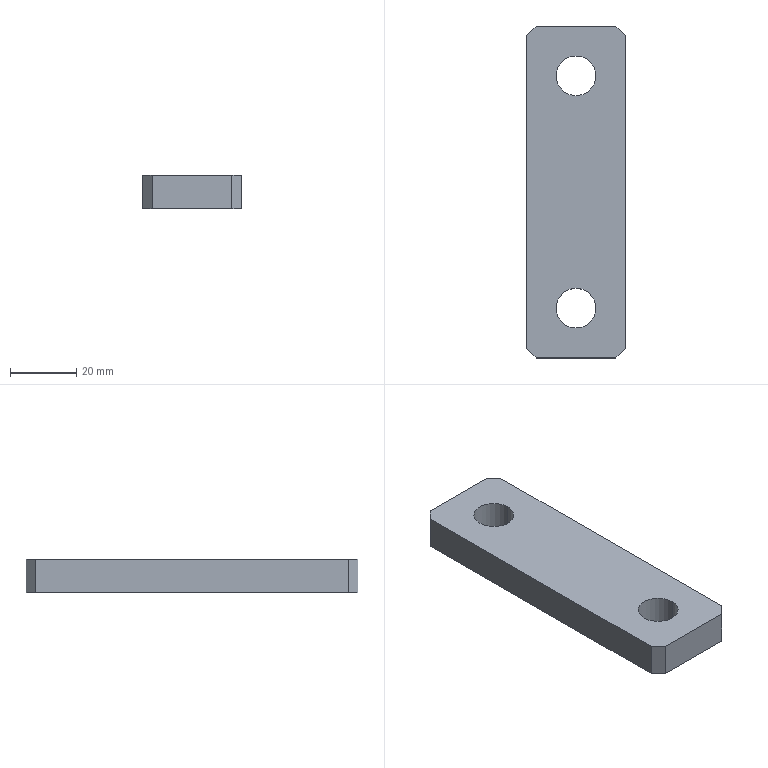Part | STEP file | 1 solid | 14 faces | box 30 x 100 x 10 mm | volume 27558 mm3 | plane 10 | cylinder 4 | commonest cylinder face diameters 12 x4
STEP:
#1=CARTESIAN_POINT('',(0.,0.,0.));
#2=DIRECTION('',(0.,0.,1.));
#3=DIRECTION('',(1.,0.,0.));
#4=AXIS2_PLACEMENT_3D('',#1,#2,#3);
#5=CARTESIAN_POINT('',(-6.,35.,5.));
#6=VERTEX_POINT('',#5);
#7=CARTESIAN_POINT('',(-6.,35.,-5.));
#8=VERTEX_POINT('',#7);
#9=CARTESIAN_POINT('',(-6.,35.,-5.));
#10=DIRECTION('',(0.,0.,-1.));
#11=VECTOR('',#10,1.);
#12=LINE('',#9,#11);
#13=CARTESIAN_POINT('',(0.,35.,-5.));
#14=DIRECTION('',(0.,0.,-1.));
#15=DIRECTION('',(-1.,0.,0.));
#16=AXIS2_PLACEMENT_3D('',#13,#14,#15);
#17=CYLINDRICAL_SURFACE('',#16,6.);
#18=CARTESIAN_POINT('',(6.283,0.));
#19=DIRECTION('',(0.,1.));
#20=VECTOR('',#19,1.);
#21=LINE('',#18,#20);
#22=(GEOMETRIC_REPRESENTATION_CONTEXT(2)PARAMETRIC_REPRESENTATION_CONTEXT()REPRESENTATION_CONTEXT('',''));
#23=DEFINITIONAL_REPRESENTATION('',(#21),#22);
#24=PCURVE('',#17,#23);
#25=CARTESIAN_POINT('',(0.,35.,-5.));
#26=DIRECTION('',(0.,0.,-1.));
#27=DIRECTION('',(-1.,0.,0.));
#28=AXIS2_PLACEMENT_3D('',#25,#26,#27);
#29=CYLINDRICAL_SURFACE('',#28,6.);
#30=CARTESIAN_POINT('',(0.,0.));
#31=DIRECTION('',(0.,1.));
#32=VECTOR('',#31,1.);
#33=LINE('',#30,#32);
#34=(GEOMETRIC_REPRESENTATION_CONTEXT(2)PARAMETRIC_REPRESENTATION_CONTEXT()REPRESENTATION_CONTEXT('',''));
#35=DEFINITIONAL_REPRESENTATION('',(#33),#34);
#36=PCURVE('',#29,#35);
#37=SURFACE_CURVE('',#12,(#24,#36),.PCURVE_S1.);
#38=EDGE_CURVE('',#6,#8,#37,.T.);
#39=ORIENTED_EDGE('',*,*,#38,.T.);
#40=CARTESIAN_POINT('',(6.,35.,-5.));
#41=VERTEX_POINT('',#40);
#42=CARTESIAN_POINT('',(0.,35.,-5.));
#43=DIRECTION('',(0.,0.,1.));
#44=DIRECTION('',(-1.,0.,0.));
#45=AXIS2_PLACEMENT_3D('',#42,#43,#44);
#46=CIRCLE('',#45,6.);
#47=CARTESIAN_POINT('',(6.283,0.));
#48=DIRECTION('',(-1.,0.));
#49=VECTOR('',#48,1.);
#50=LINE('',#47,#49);
#51=(GEOMETRIC_REPRESENTATION_CONTEXT(2)PARAMETRIC_REPRESENTATION_CONTEXT()REPRESENTATION_CONTEXT('',''));
#52=DEFINITIONAL_REPRESENTATION('',(#50),#51);
#53=PCURVE('',#17,#52);
#54=CARTESIAN_POINT('',(0.,0.,-5.));
#55=DIRECTION('',(0.,0.,1.));
#56=DIRECTION('',(1.,0.,0.));
#57=AXIS2_PLACEMENT_3D('',#54,#55,#56);
#58=PLANE('',#57);
#59=CARTESIAN_POINT('',(0.,35.));
#60=DIRECTION('',(-1.,0.));
#61=AXIS2_PLACEMENT_2D('',#59,#60);
#62=CIRCLE('',#61,6.);
#63=(GEOMETRIC_REPRESENTATION_CONTEXT(2)PARAMETRIC_REPRESENTATION_CONTEXT()REPRESENTATION_CONTEXT('',''));
#64=DEFINITIONAL_REPRESENTATION('',(#62),#63);
#65=PCURVE('',#58,#64);
#66=SURFACE_CURVE('',#46,(#53,#65),.PCURVE_S1.);
#67=EDGE_CURVE('',#8,#41,#66,.T.);
#68=ORIENTED_EDGE('',*,*,#67,.T.);
#69=CARTESIAN_POINT('',(6.,35.,5.));
#70=VERTEX_POINT('',#69);
#71=CARTESIAN_POINT('',(6.,35.,-5.));
#72=DIRECTION('',(0.,0.,-1.));
#73=VECTOR('',#72,1.);
#74=LINE('',#71,#73);
#75=CARTESIAN_POINT('',(3.142,0.));
#76=DIRECTION('',(0.,1.));
#77=VECTOR('',#76,1.);
#78=LINE('',#75,#77);
#79=(GEOMETRIC_REPRESENTATION_CONTEXT(2)PARAMETRIC_REPRESENTATION_CONTEXT()REPRESENTATION_CONTEXT('',''));
#80=DEFINITIONAL_REPRESENTATION('',(#78),#79);
#81=PCURVE('',#17,#80);
#82=CARTESIAN_POINT('',(3.142,0.));
#83=DIRECTION('',(0.,1.));
#84=VECTOR('',#83,1.);
#85=LINE('',#82,#84);
#86=(GEOMETRIC_REPRESENTATION_CONTEXT(2)PARAMETRIC_REPRESENTATION_CONTEXT()REPRESENTATION_CONTEXT('',''));
#87=DEFINITIONAL_REPRESENTATION('',(#85),#86);
#88=PCURVE('',#29,#87);
#89=SURFACE_CURVE('',#74,(#81,#88),.PCURVE_S1.);
#90=EDGE_CURVE('',#70,#41,#89,.T.);
#91=ORIENTED_EDGE('',*,*,#90,.F.);
#92=CARTESIAN_POINT('',(0.,35.,5.));
#93=DIRECTION('',(0.,0.,-1.));
#94=DIRECTION('',(-1.,0.,0.));
#95=AXIS2_PLACEMENT_3D('',#92,#93,#94);
#96=CIRCLE('',#95,6.);
#97=CARTESIAN_POINT('',(0.,-10.));
#98=DIRECTION('',(1.,0.));
#99=VECTOR('',#98,1.);
#100=LINE('',#97,#99);
#101=(GEOMETRIC_REPRESENTATION_CONTEXT(2)PARAMETRIC_REPRESENTATION_CONTEXT()REPRESENTATION_CONTEXT('',''));
#102=DEFINITIONAL_REPRESENTATION('',(#100),#101);
#103=PCURVE('',#17,#102);
#104=CARTESIAN_POINT('',(0.,0.,5.));
#105=DIRECTION('',(0.,0.,1.));
#106=DIRECTION('',(1.,0.,0.));
#107=AXIS2_PLACEMENT_3D('',#104,#105,#106);
#108=PLANE('',#107);
#109=CARTESIAN_POINT('',(-6.,35.));
#110=CARTESIAN_POINT('',(-6.,45.392));
#111=CARTESIAN_POINT('',(3.,40.196));
#112=CARTESIAN_POINT('',(12.,35.));
#113=CARTESIAN_POINT('',(3.,29.804));
#114=CARTESIAN_POINT('',(-6.,24.608));
#115=CARTESIAN_POINT('',(-6.,35.));
#116=(BOUNDED_CURVE()B_SPLINE_CURVE(2,(#109,#110,#111,#112,#113,#114,#115),.UNSPECIFIED.,.T.,.F.)B_SPLINE_CURVE_WITH_KNOTS((1,2,2,2,2,1),(-2.094,0.,2.094,4.189,6.283,8.378),.UNSPECIFIED.)CURVE()GEOMETRIC_REPRESENTATION_ITEM()RATIONAL_B_SPLINE_CURVE((1.,0.5,1.,0.5,1.,0.5,1.))REPRESENTATION_ITEM(''));
#117=(GEOMETRIC_REPRESENTATION_CONTEXT(2)PARAMETRIC_REPRESENTATION_CONTEXT()REPRESENTATION_CONTEXT('',''));
#118=DEFINITIONAL_REPRESENTATION('',(#116),#117);
#119=PCURVE('',#108,#118);
#120=SURFACE_CURVE('',#96,(#103,#119),.PCURVE_S1.);
#121=EDGE_CURVE('',#70,#6,#120,.T.);
#122=ORIENTED_EDGE('',*,*,#121,.T.);
#123=EDGE_LOOP('',(#39,#68,#91,#122));
#124=FACE_BOUND('',#123,.F.);
#125=ADVANCED_FACE('',(#124),#17,.F.);
#126=CARTESIAN_POINT('',(-6.,-35.,5.));
#127=VERTEX_POINT('',#126);
#128=CARTESIAN_POINT('',(-6.,-35.,-5.));
#129=VERTEX_POINT('',#128);
#130=CARTESIAN_POINT('',(-6.,-35.,-5.));
#131=DIRECTION('',(0.,0.,-1.));
#132=VECTOR('',#131,1.);
#133=LINE('',#130,#132);
#134=CARTESIAN_POINT('',(0.,-35.,-5.));
#135=DIRECTION('',(0.,0.,-1.));
#136=DIRECTION('',(-1.,0.,0.));
#137=AXIS2_PLACEMENT_3D('',#134,#135,#136);
#138=CYLINDRICAL_SURFACE('',#137,6.);
#139=CARTESIAN_POINT('',(6.283,0.));
#140=DIRECTION('',(0.,1.));
#141=VECTOR('',#140,1.);
#142=LINE('',#139,#141);
#143=(GEOMETRIC_REPRESENTATION_CONTEXT(2)PARAMETRIC_REPRESENTATION_CONTEXT()REPRESENTATION_CONTEXT('',''));
#144=DEFINITIONAL_REPRESENTATION('',(#142),#143);
#145=PCURVE('',#138,#144);
#146=CARTESIAN_POINT('',(0.,-35.,-5.));
#147=DIRECTION('',(0.,0.,-1.));
#148=DIRECTION('',(-1.,0.,0.));
#149=AXIS2_PLACEMENT_3D('',#146,#147,#148);
#150=CYLINDRICAL_SURFACE('',#149,6.);
#151=CARTESIAN_POINT('',(0.,0.));
#152=DIRECTION('',(0.,1.));
#153=VECTOR('',#152,1.);
#154=LINE('',#151,#153);
#155=(GEOMETRIC_REPRESENTATION_CONTEXT(2)PARAMETRIC_REPRESENTATION_CONTEXT()REPRESENTATION_CONTEXT('',''));
#156=DEFINITIONAL_REPRESENTATION('',(#154),#155);
#157=PCURVE('',#150,#156);
#158=SURFACE_CURVE('',#133,(#145,#157),.PCURVE_S1.);
#159=EDGE_CURVE('',#127,#129,#158,.T.);
#160=ORIENTED_EDGE('',*,*,#159,.T.);
#161=CARTESIAN_POINT('',(6.,-35.,-5.));
#162=VERTEX_POINT('',#161);
#163=CARTESIAN_POINT('',(0.,-35.,-5.));
#164=DIRECTION('',(0.,0.,1.));
#165=DIRECTION('',(-1.,0.,0.));
#166=AXIS2_PLACEMENT_3D('',#163,#164,#165);
#167=CIRCLE('',#166,6.);
#168=CARTESIAN_POINT('',(6.283,0.));
#169=DIRECTION('',(-1.,0.));
#170=VECTOR('',#169,1.);
#171=LINE('',#168,#170);
#172=(GEOMETRIC_REPRESENTATION_CONTEXT(2)PARAMETRIC_REPRESENTATION_CONTEXT()REPRESENTATION_CONTEXT('',''));
#173=DEFINITIONAL_REPRESENTATION('',(#171),#172);
#174=PCURVE('',#138,#173);
#175=CARTESIAN_POINT('',(0.,-35.));
#176=DIRECTION('',(-1.,0.));
#177=AXIS2_PLACEMENT_2D('',#175,#176);
#178=CIRCLE('',#177,6.);
#179=(GEOMETRIC_REPRESENTATION_CONTEXT(2)PARAMETRIC_REPRESENTATION_CONTEXT()REPRESENTATION_CONTEXT('',''));
#180=DEFINITIONAL_REPRESENTATION('',(#178),#179);
#181=PCURVE('',#58,#180);
#182=SURFACE_CURVE('',#167,(#174,#181),.PCURVE_S1.);
#183=EDGE_CURVE('',#129,#162,#182,.T.);
#184=ORIENTED_EDGE('',*,*,#183,.T.);
#185=CARTESIAN_POINT('',(6.,-35.,5.));
#186=VERTEX_POINT('',#185);
#187=CARTESIAN_POINT('',(6.,-35.,-5.));
#188=DIRECTION('',(0.,0.,-1.));
#189=VECTOR('',#188,1.);
#190=LINE('',#187,#189);
#191=CARTESIAN_POINT('',(3.142,0.));
#192=DIRECTION('',(0.,1.));
#193=VECTOR('',#192,1.);
#194=LINE('',#191,#193);
#195=(GEOMETRIC_REPRESENTATION_CONTEXT(2)PARAMETRIC_REPRESENTATION_CONTEXT()REPRESENTATION_CONTEXT('',''));
#196=DEFINITIONAL_REPRESENTATION('',(#194),#195);
#197=PCURVE('',#138,#196);
#198=CARTESIAN_POINT('',(3.142,0.));
#199=DIRECTION('',(0.,1.));
#200=VECTOR('',#199,1.);
#201=LINE('',#198,#200);
#202=(GEOMETRIC_REPRESENTATION_CONTEXT(2)PARAMETRIC_REPRESENTATION_CONTEXT()REPRESENTATION_CONTEXT('',''));
#203=DEFINITIONAL_REPRESENTATION('',(#201),#202);
#204=PCURVE('',#150,#203);
#205=SURFACE_CURVE('',#190,(#197,#204),.PCURVE_S1.);
#206=EDGE_CURVE('',#186,#162,#205,.T.);
#207=ORIENTED_EDGE('',*,*,#206,.F.);
#208=CARTESIAN_POINT('',(0.,-35.,5.));
#209=DIRECTION('',(0.,0.,-1.));
#210=DIRECTION('',(-1.,0.,0.));
#211=AXIS2_PLACEMENT_3D('',#208,#209,#210);
#212=CIRCLE('',#211,6.);
#213=CARTESIAN_POINT('',(0.,-10.));
#214=DIRECTION('',(1.,0.));
#215=VECTOR('',#214,1.);
#216=LINE('',#213,#215);
#217=(GEOMETRIC_REPRESENTATION_CONTEXT(2)PARAMETRIC_REPRESENTATION_CONTEXT()REPRESENTATION_CONTEXT('',''));
#218=DEFINITIONAL_REPRESENTATION('',(#216),#217);
#219=PCURVE('',#138,#218);
#220=CARTESIAN_POINT('',(-6.,-35.));
#221=CARTESIAN_POINT('',(-6.,-24.608));
#222=CARTESIAN_POINT('',(3.,-29.804));
#223=CARTESIAN_POINT('',(12.,-35.));
#224=CARTESIAN_POINT('',(3.,-40.196));
#225=CARTESIAN_POINT('',(-6.,-45.392));
#226=CARTESIAN_POINT('',(-6.,-35.));
#227=(BOUNDED_CURVE()B_SPLINE_CURVE(2,(#220,#221,#222,#223,#224,#225,#226),.UNSPECIFIED.,.T.,.F.)B_SPLINE_CURVE_WITH_KNOTS((1,2,2,2,2,1),(-2.094,0.,2.094,4.189,6.283,8.378),.UNSPECIFIED.)CURVE()GEOMETRIC_REPRESENTATION_ITEM()RATIONAL_B_SPLINE_CURVE((1.,0.5,1.,0.5,1.,0.5,1.))REPRESENTATION_ITEM(''));
#228=(GEOMETRIC_REPRESENTATION_CONTEXT(2)PARAMETRIC_REPRESENTATION_CONTEXT()REPRESENTATION_CONTEXT('',''));
#229=DEFINITIONAL_REPRESENTATION('',(#227),#228);
#230=PCURVE('',#108,#229);
#231=SURFACE_CURVE('',#212,(#219,#230),.PCURVE_S1.);
#232=EDGE_CURVE('',#186,#127,#231,.T.);
#233=ORIENTED_EDGE('',*,*,#232,.T.);
#234=EDGE_LOOP('',(#160,#184,#207,#233));
#235=FACE_BOUND('',#234,.F.);
#236=ADVANCED_FACE('',(#235),#138,.F.);
#237=CARTESIAN_POINT('',(0.,35.,5.));
#238=DIRECTION('',(0.,0.,-1.));
#239=DIRECTION('',(-1.,0.,0.));
#240=AXIS2_PLACEMENT_3D('',#237,#238,#239);
#241=CIRCLE('',#240,6.);
#242=CARTESIAN_POINT('',(-6.,35.));
#243=CARTESIAN_POINT('',(-6.,45.392));
#244=CARTESIAN_POINT('',(3.,40.196));
#245=CARTESIAN_POINT('',(12.,35.));
#246=CARTESIAN_POINT('',(3.,29.804));
#247=CARTESIAN_POINT('',(-6.,24.608));
#248=CARTESIAN_POINT('',(-6.,35.));
#249=(BOUNDED_CURVE()B_SPLINE_CURVE(2,(#242,#243,#244,#245,#246,#247,#248),.UNSPECIFIED.,.T.,.F.)B_SPLINE_CURVE_WITH_KNOTS((1,2,2,2,2,1),(-2.094,0.,2.094,4.189,6.283,8.378),.UNSPECIFIED.)CURVE()GEOMETRIC_REPRESENTATION_ITEM()RATIONAL_B_SPLINE_CURVE((1.,0.5,1.,0.5,1.,0.5,1.))REPRESENTATION_ITEM(''));
#250=(GEOMETRIC_REPRESENTATION_CONTEXT(2)PARAMETRIC_REPRESENTATION_CONTEXT()REPRESENTATION_CONTEXT('',''));
#251=DEFINITIONAL_REPRESENTATION('',(#249),#250);
#252=PCURVE('',#108,#251);
#253=CARTESIAN_POINT('',(0.,-10.));
#254=DIRECTION('',(1.,0.));
#255=VECTOR('',#254,1.);
#256=LINE('',#253,#255);
#257=(GEOMETRIC_REPRESENTATION_CONTEXT(2)PARAMETRIC_REPRESENTATION_CONTEXT()REPRESENTATION_CONTEXT('',''));
#258=DEFINITIONAL_REPRESENTATION('',(#256),#257);
#259=PCURVE('',#29,#258);
#260=SURFACE_CURVE('',#241,(#252,#259),.PCURVE_S1.);
#261=EDGE_CURVE('',#6,#70,#260,.T.);
#262=ORIENTED_EDGE('',*,*,#261,.T.);
#263=ORIENTED_EDGE('',*,*,#121,.T.);
#264=EDGE_LOOP('',(#262,#263));
#265=FACE_BOUND('',#264,.T.);
#266=CARTESIAN_POINT('',(0.,-35.,5.));
#267=DIRECTION('',(0.,0.,-1.));
#268=DIRECTION('',(-1.,0.,0.));
#269=AXIS2_PLACEMENT_3D('',#266,#267,#268);
#270=CIRCLE('',#269,6.);
#271=CARTESIAN_POINT('',(-6.,-35.));
#272=CARTESIAN_POINT('',(-6.,-24.608));
#273=CARTESIAN_POINT('',(3.,-29.804));
#274=CARTESIAN_POINT('',(12.,-35.));
#275=CARTESIAN_POINT('',(3.,-40.196));
#276=CARTESIAN_POINT('',(-6.,-45.392));
#277=CARTESIAN_POINT('',(-6.,-35.));
#278=(BOUNDED_CURVE()B_SPLINE_CURVE(2,(#271,#272,#273,#274,#275,#276,#277),.UNSPECIFIED.,.T.,.F.)B_SPLINE_CURVE_WITH_KNOTS((1,2,2,2,2,1),(-2.094,0.,2.094,4.189,6.283,8.378),.UNSPECIFIED.)CURVE()GEOMETRIC_REPRESENTATION_ITEM()RATIONAL_B_SPLINE_CURVE((1.,0.5,1.,0.5,1.,0.5,1.))REPRESENTATION_ITEM(''));
#279=(GEOMETRIC_REPRESENTATION_CONTEXT(2)PARAMETRIC_REPRESENTATION_CONTEXT()REPRESENTATION_CONTEXT('',''));
#280=DEFINITIONAL_REPRESENTATION('',(#278),#279);
#281=PCURVE('',#108,#280);
#282=CARTESIAN_POINT('',(0.,-10.));
#283=DIRECTION('',(1.,0.));
#284=VECTOR('',#283,1.);
#285=LINE('',#282,#284);
#286=(GEOMETRIC_REPRESENTATION_CONTEXT(2)PARAMETRIC_REPRESENTATION_CONTEXT()REPRESENTATION_CONTEXT('',''));
#287=DEFINITIONAL_REPRESENTATION('',(#285),#286);
#288=PCURVE('',#150,#287);
#289=SURFACE_CURVE('',#270,(#281,#288),.PCURVE_S1.);
#290=EDGE_CURVE('',#127,#186,#289,.T.);
#291=ORIENTED_EDGE('',*,*,#290,.T.);
#292=ORIENTED_EDGE('',*,*,#232,.T.);
#293=EDGE_LOOP('',(#291,#292));
#294=FACE_BOUND('',#293,.T.);
#295=CARTESIAN_POINT('',(12.,50.,5.));
#296=VERTEX_POINT('',#295);
#297=CARTESIAN_POINT('',(-12.,50.,5.));
#298=VERTEX_POINT('',#297);
#299=CARTESIAN_POINT('',(0.,50.,5.));
#300=DIRECTION('',(-1.,0.,0.));
#301=VECTOR('',#300,1.);
#302=LINE('',#299,#301);
#303=CARTESIAN_POINT('',(0.,50.));
#304=DIRECTION('',(-1.,0.));
#305=VECTOR('',#304,1.);
#306=LINE('',#303,#305);
#307=(GEOMETRIC_REPRESENTATION_CONTEXT(2)PARAMETRIC_REPRESENTATION_CONTEXT()REPRESENTATION_CONTEXT('',''));
#308=DEFINITIONAL_REPRESENTATION('',(#306),#307);
#309=PCURVE('',#108,#308);
#310=CARTESIAN_POINT('',(-15.,50.,5.));
#311=DIRECTION('',(0.,-1.,0.));
#312=DIRECTION('',(0.,0.,-1.));
#313=AXIS2_PLACEMENT_3D('',#310,#311,#312);
#314=PLANE('',#313);
#315=CARTESIAN_POINT('',(0.,15.));
#316=DIRECTION('',(0.,-1.));
#317=VECTOR('',#316,1.);
#318=LINE('',#315,#317);
#319=(GEOMETRIC_REPRESENTATION_CONTEXT(2)PARAMETRIC_REPRESENTATION_CONTEXT()REPRESENTATION_CONTEXT('',''));
#320=DEFINITIONAL_REPRESENTATION('',(#318),#319);
#321=PCURVE('',#314,#320);
#322=SURFACE_CURVE('',#302,(#309,#321),.PCURVE_S1.);
#323=EDGE_CURVE('',#296,#298,#322,.T.);
#324=ORIENTED_EDGE('',*,*,#323,.T.);
#325=CARTESIAN_POINT('',(-15.,47.,5.));
#326=VERTEX_POINT('',#325);
#327=CARTESIAN_POINT('',(-12.,50.,5.));
#328=DIRECTION('',(-0.7071,-0.7071,0.));
#329=VECTOR('',#328,1.);
#330=LINE('',#327,#329);
#331=CARTESIAN_POINT('',(-12.,50.));
#332=DIRECTION('',(-0.7071,-0.7071));
#333=VECTOR('',#332,1.);
#334=LINE('',#331,#333);
#335=(GEOMETRIC_REPRESENTATION_CONTEXT(2)PARAMETRIC_REPRESENTATION_CONTEXT()REPRESENTATION_CONTEXT('',''));
#336=DEFINITIONAL_REPRESENTATION('',(#334),#335);
#337=PCURVE('',#108,#336);
#338=CARTESIAN_POINT('',(-15.,47.,5.));
#339=DIRECTION('',(0.7071,-0.7071,0.));
#340=DIRECTION('',(0.7071,0.7071,0.));
#341=AXIS2_PLACEMENT_3D('',#338,#339,#340);
#342=PLANE('',#341);
#343=CARTESIAN_POINT('',(4.243,0.));
#344=DIRECTION('',(-1.,0.));
#345=VECTOR('',#344,1.);
#346=LINE('',#343,#345);
#347=(GEOMETRIC_REPRESENTATION_CONTEXT(2)PARAMETRIC_REPRESENTATION_CONTEXT()REPRESENTATION_CONTEXT('',''));
#348=DEFINITIONAL_REPRESENTATION('',(#346),#347);
#349=PCURVE('',#342,#348);
#350=SURFACE_CURVE('',#330,(#337,#349),.PCURVE_S1.);
#351=EDGE_CURVE('',#298,#326,#350,.T.);
#352=ORIENTED_EDGE('',*,*,#351,.T.);
#353=CARTESIAN_POINT('',(-15.,-47.,5.));
#354=VERTEX_POINT('',#353);
#355=CARTESIAN_POINT('',(-15.,0.,5.));
#356=DIRECTION('',(0.,-1.,0.));
#357=VECTOR('',#356,1.);
#358=LINE('',#355,#357);
#359=CARTESIAN_POINT('',(-15.,0.));
#360=DIRECTION('',(0.,-1.));
#361=VECTOR('',#360,1.);
#362=LINE('',#359,#361);
#363=(GEOMETRIC_REPRESENTATION_CONTEXT(2)PARAMETRIC_REPRESENTATION_CONTEXT()REPRESENTATION_CONTEXT('',''));
#364=DEFINITIONAL_REPRESENTATION('',(#362),#363);
#365=PCURVE('',#108,#364);
#366=CARTESIAN_POINT('',(-15.,50.,5.));
#367=DIRECTION('',(1.,0.,0.));
#368=DIRECTION('',(0.,1.,0.));
#369=AXIS2_PLACEMENT_3D('',#366,#367,#368);
#370=PLANE('',#369);
#371=CARTESIAN_POINT('',(-50.,0.));
#372=DIRECTION('',(-1.,0.));
#373=VECTOR('',#372,1.);
#374=LINE('',#371,#373);
#375=(GEOMETRIC_REPRESENTATION_CONTEXT(2)PARAMETRIC_REPRESENTATION_CONTEXT()REPRESENTATION_CONTEXT('',''));
#376=DEFINITIONAL_REPRESENTATION('',(#374),#375);
#377=PCURVE('',#370,#376);
#378=SURFACE_CURVE('',#358,(#365,#377),.PCURVE_S1.);
#379=EDGE_CURVE('',#326,#354,#378,.T.);
#380=ORIENTED_EDGE('',*,*,#379,.T.);
#381=CARTESIAN_POINT('',(-12.,-50.,5.));
#382=VERTEX_POINT('',#381);
#383=CARTESIAN_POINT('',(-15.,-47.,5.));
#384=DIRECTION('',(0.7071,-0.7071,0.));
#385=VECTOR('',#384,1.);
#386=LINE('',#383,#385);
#387=CARTESIAN_POINT('',(-15.,-47.));
#388=DIRECTION('',(0.7071,-0.7071));
#389=VECTOR('',#388,1.);
#390=LINE('',#387,#389);
#391=(GEOMETRIC_REPRESENTATION_CONTEXT(2)PARAMETRIC_REPRESENTATION_CONTEXT()REPRESENTATION_CONTEXT('',''));
#392=DEFINITIONAL_REPRESENTATION('',(#390),#391);
#393=PCURVE('',#108,#392);
#394=CARTESIAN_POINT('',(-12.,-50.,5.));
#395=DIRECTION('',(0.7071,0.7071,0.));
#396=DIRECTION('',(-0.7071,0.7071,0.));
#397=AXIS2_PLACEMENT_3D('',#394,#395,#396);
#398=PLANE('',#397);
#399=CARTESIAN_POINT('',(4.243,0.));
#400=DIRECTION('',(-1.,0.));
#401=VECTOR('',#400,1.);
#402=LINE('',#399,#401);
#403=(GEOMETRIC_REPRESENTATION_CONTEXT(2)PARAMETRIC_REPRESENTATION_CONTEXT()REPRESENTATION_CONTEXT('',''));
#404=DEFINITIONAL_REPRESENTATION('',(#402),#403);
#405=PCURVE('',#398,#404);
#406=SURFACE_CURVE('',#386,(#393,#405),.PCURVE_S1.);
#407=EDGE_CURVE('',#354,#382,#406,.T.);
#408=ORIENTED_EDGE('',*,*,#407,.T.);
#409=CARTESIAN_POINT('',(12.,-50.,5.));
#410=VERTEX_POINT('',#409);
#411=CARTESIAN_POINT('',(0.,-50.,5.));
#412=DIRECTION('',(1.,0.,0.));
#413=VECTOR('',#412,1.);
#414=LINE('',#411,#413);
#415=CARTESIAN_POINT('',(0.,-50.));
#416=DIRECTION('',(1.,0.));
#417=VECTOR('',#416,1.);
#418=LINE('',#415,#417);
#419=(GEOMETRIC_REPRESENTATION_CONTEXT(2)PARAMETRIC_REPRESENTATION_CONTEXT()REPRESENTATION_CONTEXT('',''));
#420=DEFINITIONAL_REPRESENTATION('',(#418),#419);
#421=PCURVE('',#108,#420);
#422=CARTESIAN_POINT('',(-15.,-50.,5.));
#423=DIRECTION('',(0.,1.,0.));
#424=DIRECTION('',(0.,0.,1.));
#425=AXIS2_PLACEMENT_3D('',#422,#423,#424);
#426=PLANE('',#425);
#427=CARTESIAN_POINT('',(0.,15.));
#428=DIRECTION('',(0.,1.));
#429=VECTOR('',#428,1.);
#430=LINE('',#427,#429);
#431=(GEOMETRIC_REPRESENTATION_CONTEXT(2)PARAMETRIC_REPRESENTATION_CONTEXT()REPRESENTATION_CONTEXT('',''));
#432=DEFINITIONAL_REPRESENTATION('',(#430),#431);
#433=PCURVE('',#426,#432);
#434=SURFACE_CURVE('',#414,(#421,#433),.PCURVE_S1.);
#435=EDGE_CURVE('',#382,#410,#434,.T.);
#436=ORIENTED_EDGE('',*,*,#435,.T.);
#437=CARTESIAN_POINT('',(15.,-47.,5.));
#438=VERTEX_POINT('',#437);
#439=CARTESIAN_POINT('',(12.,-50.,5.));
#440=DIRECTION('',(0.7071,0.7071,0.));
#441=VECTOR('',#440,1.);
#442=LINE('',#439,#441);
#443=CARTESIAN_POINT('',(12.,-50.));
#444=DIRECTION('',(0.7071,0.7071));
#445=VECTOR('',#444,1.);
#446=LINE('',#443,#445);
#447=(GEOMETRIC_REPRESENTATION_CONTEXT(2)PARAMETRIC_REPRESENTATION_CONTEXT()REPRESENTATION_CONTEXT('',''));
#448=DEFINITIONAL_REPRESENTATION('',(#446),#447);
#449=PCURVE('',#108,#448);
#450=CARTESIAN_POINT('',(15.,-47.,5.));
#451=DIRECTION('',(-0.7071,0.7071,0.));
#452=DIRECTION('',(-0.7071,-0.7071,0.));
#453=AXIS2_PLACEMENT_3D('',#450,#451,#452);
#454=PLANE('',#453);
#455=CARTESIAN_POINT('',(4.243,0.));
#456=DIRECTION('',(-1.,0.));
#457=VECTOR('',#456,1.);
#458=LINE('',#455,#457);
#459=(GEOMETRIC_REPRESENTATION_CONTEXT(2)PARAMETRIC_REPRESENTATION_CONTEXT()REPRESENTATION_CONTEXT('',''));
#460=DEFINITIONAL_REPRESENTATION('',(#458),#459);
#461=PCURVE('',#454,#460);
#462=SURFACE_CURVE('',#442,(#449,#461),.PCURVE_S1.);
#463=EDGE_CURVE('',#410,#438,#462,.T.);
#464=ORIENTED_EDGE('',*,*,#463,.T.);
#465=CARTESIAN_POINT('',(15.,47.,5.));
#466=VERTEX_POINT('',#465);
#467=CARTESIAN_POINT('',(15.,0.,5.));
#468=DIRECTION('',(0.,1.,0.));
#469=VECTOR('',#468,1.);
#470=LINE('',#467,#469);
#471=CARTESIAN_POINT('',(15.,0.));
#472=DIRECTION('',(0.,1.));
#473=VECTOR('',#472,1.);
#474=LINE('',#471,#473);
#475=(GEOMETRIC_REPRESENTATION_CONTEXT(2)PARAMETRIC_REPRESENTATION_CONTEXT()REPRESENTATION_CONTEXT('',''));
#476=DEFINITIONAL_REPRESENTATION('',(#474),#475);
#477=PCURVE('',#108,#476);
#478=CARTESIAN_POINT('',(15.,50.,5.));
#479=DIRECTION('',(-1.,0.,0.));
#480=DIRECTION('',(0.,-1.,0.));
#481=AXIS2_PLACEMENT_3D('',#478,#479,#480);
#482=PLANE('',#481);
#483=CARTESIAN_POINT('',(50.,0.));
#484=DIRECTION('',(-1.,0.));
#485=VECTOR('',#484,1.);
#486=LINE('',#483,#485);
#487=(GEOMETRIC_REPRESENTATION_CONTEXT(2)PARAMETRIC_REPRESENTATION_CONTEXT()REPRESENTATION_CONTEXT('',''));
#488=DEFINITIONAL_REPRESENTATION('',(#486),#487);
#489=PCURVE('',#482,#488);
#490=SURFACE_CURVE('',#470,(#477,#489),.PCURVE_S1.);
#491=EDGE_CURVE('',#438,#466,#490,.T.);
#492=ORIENTED_EDGE('',*,*,#491,.T.);
#493=CARTESIAN_POINT('',(15.,47.,5.));
#494=DIRECTION('',(-0.7071,0.7071,0.));
#495=VECTOR('',#494,1.);
#496=LINE('',#493,#495);
#497=CARTESIAN_POINT('',(15.,47.));
#498=DIRECTION('',(-0.7071,0.7071));
#499=VECTOR('',#498,1.);
#500=LINE('',#497,#499);
#501=(GEOMETRIC_REPRESENTATION_CONTEXT(2)PARAMETRIC_REPRESENTATION_CONTEXT()REPRESENTATION_CONTEXT('',''));
#502=DEFINITIONAL_REPRESENTATION('',(#500),#501);
#503=PCURVE('',#108,#502);
#504=CARTESIAN_POINT('',(12.,50.,5.));
#505=DIRECTION('',(-0.7071,-0.7071,0.));
#506=DIRECTION('',(0.7071,-0.7071,0.));
#507=AXIS2_PLACEMENT_3D('',#504,#505,#506);
#508=PLANE('',#507);
#509=CARTESIAN_POINT('',(4.243,0.));
#510=DIRECTION('',(-1.,0.));
#511=VECTOR('',#510,1.);
#512=LINE('',#509,#511);
#513=(GEOMETRIC_REPRESENTATION_CONTEXT(2)PARAMETRIC_REPRESENTATION_CONTEXT()REPRESENTATION_CONTEXT('',''));
#514=DEFINITIONAL_REPRESENTATION('',(#512),#513);
#515=PCURVE('',#508,#514);
#516=SURFACE_CURVE('',#496,(#503,#515),.PCURVE_S1.);
#517=EDGE_CURVE('',#466,#296,#516,.T.);
#518=ORIENTED_EDGE('',*,*,#517,.T.);
#519=EDGE_LOOP('',(#324,#352,#380,#408,#436,#464,#492,#518));
#520=FACE_BOUND('',#519,.T.);
#521=ADVANCED_FACE('',(#265,#294,#520),#108,.T.);
#522=CARTESIAN_POINT('',(0.,35.,-5.));
#523=DIRECTION('',(0.,0.,1.));
#524=DIRECTION('',(-1.,0.,0.));
#525=AXIS2_PLACEMENT_3D('',#522,#523,#524);
#526=CIRCLE('',#525,6.);
#527=CARTESIAN_POINT('',(6.283,0.));
#528=DIRECTION('',(-1.,0.));
#529=VECTOR('',#528,1.);
#530=LINE('',#527,#529);
#531=(GEOMETRIC_REPRESENTATION_CONTEXT(2)PARAMETRIC_REPRESENTATION_CONTEXT()REPRESENTATION_CONTEXT('',''));
#532=DEFINITIONAL_REPRESENTATION('',(#530),#531);
#533=PCURVE('',#29,#532);
#534=CARTESIAN_POINT('',(0.,35.));
#535=DIRECTION('',(-1.,0.));
#536=AXIS2_PLACEMENT_2D('',#534,#535);
#537=CIRCLE('',#536,6.);
#538=(GEOMETRIC_REPRESENTATION_CONTEXT(2)PARAMETRIC_REPRESENTATION_CONTEXT()REPRESENTATION_CONTEXT('',''));
#539=DEFINITIONAL_REPRESENTATION('',(#537),#538);
#540=PCURVE('',#58,#539);
#541=SURFACE_CURVE('',#526,(#533,#540),.PCURVE_S1.);
#542=EDGE_CURVE('',#41,#8,#541,.T.);
#543=ORIENTED_EDGE('',*,*,#542,.T.);
#544=ORIENTED_EDGE('',*,*,#38,.F.);
#545=ORIENTED_EDGE('',*,*,#261,.T.);
#546=ORIENTED_EDGE('',*,*,#90,.T.);
#547=EDGE_LOOP('',(#543,#544,#545,#546));
#548=FACE_BOUND('',#547,.F.);
#549=ADVANCED_FACE('',(#548),#29,.F.);
#550=CARTESIAN_POINT('',(0.,-35.,-5.));
#551=DIRECTION('',(0.,0.,1.));
#552=DIRECTION('',(-1.,0.,0.));
#553=AXIS2_PLACEMENT_3D('',#550,#551,#552);
#554=CIRCLE('',#553,6.);
#555=CARTESIAN_POINT('',(6.283,0.));
#556=DIRECTION('',(-1.,0.));
#557=VECTOR('',#556,1.);
#558=LINE('',#555,#557);
#559=(GEOMETRIC_REPRESENTATION_CONTEXT(2)PARAMETRIC_REPRESENTATION_CONTEXT()REPRESENTATION_CONTEXT('',''));
#560=DEFINITIONAL_REPRESENTATION('',(#558),#559);
#561=PCURVE('',#150,#560);
#562=CARTESIAN_POINT('',(0.,-35.));
#563=DIRECTION('',(-1.,0.));
#564=AXIS2_PLACEMENT_2D('',#562,#563);
#565=CIRCLE('',#564,6.);
#566=(GEOMETRIC_REPRESENTATION_CONTEXT(2)PARAMETRIC_REPRESENTATION_CONTEXT()REPRESENTATION_CONTEXT('',''));
#567=DEFINITIONAL_REPRESENTATION('',(#565),#566);
#568=PCURVE('',#58,#567);
#569=SURFACE_CURVE('',#554,(#561,#568),.PCURVE_S1.);
#570=EDGE_CURVE('',#162,#129,#569,.T.);
#571=ORIENTED_EDGE('',*,*,#570,.T.);
#572=ORIENTED_EDGE('',*,*,#159,.F.);
#573=ORIENTED_EDGE('',*,*,#290,.T.);
#574=ORIENTED_EDGE('',*,*,#206,.T.);
#575=EDGE_LOOP('',(#571,#572,#573,#574));
#576=FACE_BOUND('',#575,.F.);
#577=ADVANCED_FACE('',(#576),#150,.F.);
#578=CARTESIAN_POINT('',(-12.,50.,-5.));
#579=VERTEX_POINT('',#578);
#580=CARTESIAN_POINT('',(-12.,50.,5.));
#581=DIRECTION('',(0.,0.,1.));
#582=VECTOR('',#581,1.);
#583=LINE('',#580,#582);
#584=CARTESIAN_POINT('',(4.243,0.));
#585=DIRECTION('',(0.,1.));
#586=VECTOR('',#585,1.);
#587=LINE('',#584,#586);
#588=(GEOMETRIC_REPRESENTATION_CONTEXT(2)PARAMETRIC_REPRESENTATION_CONTEXT()REPRESENTATION_CONTEXT('',''));
#589=DEFINITIONAL_REPRESENTATION('',(#587),#588);
#590=PCURVE('',#342,#589);
#591=CARTESIAN_POINT('',(0.,3.));
#592=DIRECTION('',(-1.,0.));
#593=VECTOR('',#592,1.);
#594=LINE('',#591,#593);
#595=(GEOMETRIC_REPRESENTATION_CONTEXT(2)PARAMETRIC_REPRESENTATION_CONTEXT()REPRESENTATION_CONTEXT('',''));
#596=DEFINITIONAL_REPRESENTATION('',(#594),#595);
#597=PCURVE('',#314,#596);
#598=SURFACE_CURVE('',#583,(#590,#597),.PCURVE_S1.);
#599=EDGE_CURVE('',#579,#298,#598,.T.);
#600=ORIENTED_EDGE('',*,*,#599,.F.);
#601=CARTESIAN_POINT('',(-15.,47.,-5.));
#602=VERTEX_POINT('',#601);
#603=CARTESIAN_POINT('',(-15.,47.,-5.));
#604=DIRECTION('',(0.7071,0.7071,0.));
#605=VECTOR('',#604,1.);
#606=LINE('',#603,#605);
#607=CARTESIAN_POINT('',(0.,-10.));
#608=DIRECTION('',(1.,0.));
#609=VECTOR('',#608,1.);
#610=LINE('',#607,#609);
#611=(GEOMETRIC_REPRESENTATION_CONTEXT(2)PARAMETRIC_REPRESENTATION_CONTEXT()REPRESENTATION_CONTEXT('',''));
#612=DEFINITIONAL_REPRESENTATION('',(#610),#611);
#613=PCURVE('',#342,#612);
#614=CARTESIAN_POINT('',(-15.,47.));
#615=DIRECTION('',(0.7071,0.7071));
#616=VECTOR('',#615,1.);
#617=LINE('',#614,#616);
#618=(GEOMETRIC_REPRESENTATION_CONTEXT(2)PARAMETRIC_REPRESENTATION_CONTEXT()REPRESENTATION_CONTEXT('',''));
#619=DEFINITIONAL_REPRESENTATION('',(#617),#618);
#620=PCURVE('',#58,#619);
#621=SURFACE_CURVE('',#606,(#613,#620),.PCURVE_S1.);
#622=EDGE_CURVE('',#602,#579,#621,.T.);
#623=ORIENTED_EDGE('',*,*,#622,.F.);
#624=CARTESIAN_POINT('',(-15.,47.,5.));
#625=DIRECTION('',(0.,0.,-1.));
#626=VECTOR('',#625,1.);
#627=LINE('',#624,#626);
#628=CARTESIAN_POINT('',(0.,0.));
#629=DIRECTION('',(0.,-1.));
#630=VECTOR('',#629,1.);
#631=LINE('',#628,#630);
#632=(GEOMETRIC_REPRESENTATION_CONTEXT(2)PARAMETRIC_REPRESENTATION_CONTEXT()REPRESENTATION_CONTEXT('',''));
#633=DEFINITIONAL_REPRESENTATION('',(#631),#632);
#634=PCURVE('',#342,#633);
#635=CARTESIAN_POINT('',(-3.,0.));
#636=DIRECTION('',(0.,-1.));
#637=VECTOR('',#636,1.);
#638=LINE('',#635,#637);
#639=(GEOMETRIC_REPRESENTATION_CONTEXT(2)PARAMETRIC_REPRESENTATION_CONTEXT()REPRESENTATION_CONTEXT('',''));
#640=DEFINITIONAL_REPRESENTATION('',(#638),#639);
#641=PCURVE('',#370,#640);
#642=SURFACE_CURVE('',#627,(#634,#641),.PCURVE_S1.);
#643=EDGE_CURVE('',#326,#602,#642,.T.);
#644=ORIENTED_EDGE('',*,*,#643,.F.);
#645=ORIENTED_EDGE('',*,*,#351,.F.);
#646=EDGE_LOOP('',(#600,#623,#644,#645));
#647=FACE_BOUND('',#646,.T.);
#648=ADVANCED_FACE('',(#647),#342,.F.);
#649=ORIENTED_EDGE('',*,*,#599,.T.);
#650=ORIENTED_EDGE('',*,*,#323,.F.);
#651=CARTESIAN_POINT('',(12.,50.,-5.));
#652=VERTEX_POINT('',#651);
#653=CARTESIAN_POINT('',(12.,50.,5.));
#654=DIRECTION('',(0.,0.,1.));
#655=VECTOR('',#654,1.);
#656=LINE('',#653,#655);
#657=CARTESIAN_POINT('',(0.,27.));
#658=DIRECTION('',(-1.,0.));
#659=VECTOR('',#658,1.);
#660=LINE('',#657,#659);
#661=(GEOMETRIC_REPRESENTATION_CONTEXT(2)PARAMETRIC_REPRESENTATION_CONTEXT()REPRESENTATION_CONTEXT('',''));
#662=DEFINITIONAL_REPRESENTATION('',(#660),#661);
#663=PCURVE('',#314,#662);
#664=CARTESIAN_POINT('',(0.,0.));
#665=DIRECTION('',(0.,1.));
#666=VECTOR('',#665,1.);
#667=LINE('',#664,#666);
#668=(GEOMETRIC_REPRESENTATION_CONTEXT(2)PARAMETRIC_REPRESENTATION_CONTEXT()REPRESENTATION_CONTEXT('',''));
#669=DEFINITIONAL_REPRESENTATION('',(#667),#668);
#670=PCURVE('',#508,#669);
#671=SURFACE_CURVE('',#656,(#663,#670),.PCURVE_S1.);
#672=EDGE_CURVE('',#652,#296,#671,.T.);
#673=ORIENTED_EDGE('',*,*,#672,.F.);
#674=CARTESIAN_POINT('',(-15.,50.,-5.));
#675=DIRECTION('',(1.,0.,0.));
#676=VECTOR('',#675,1.);
#677=LINE('',#674,#676);
#678=CARTESIAN_POINT('',(10.,0.));
#679=DIRECTION('',(0.,1.));
#680=VECTOR('',#679,1.);
#681=LINE('',#678,#680);
#682=(GEOMETRIC_REPRESENTATION_CONTEXT(2)PARAMETRIC_REPRESENTATION_CONTEXT()REPRESENTATION_CONTEXT('',''));
#683=DEFINITIONAL_REPRESENTATION('',(#681),#682);
#684=PCURVE('',#314,#683);
#685=CARTESIAN_POINT('',(-15.,50.));
#686=DIRECTION('',(1.,0.));
#687=VECTOR('',#686,1.);
#688=LINE('',#685,#687);
#689=(GEOMETRIC_REPRESENTATION_CONTEXT(2)PARAMETRIC_REPRESENTATION_CONTEXT()REPRESENTATION_CONTEXT('',''));
#690=DEFINITIONAL_REPRESENTATION('',(#688),#689);
#691=PCURVE('',#58,#690);
#692=SURFACE_CURVE('',#677,(#684,#691),.PCURVE_S1.);
#693=EDGE_CURVE('',#579,#652,#692,.T.);
#694=ORIENTED_EDGE('',*,*,#693,.F.);
#695=EDGE_LOOP('',(#649,#650,#673,#694));
#696=FACE_BOUND('',#695,.T.);
#697=ADVANCED_FACE('',(#696),#314,.F.);
#698=CARTESIAN_POINT('',(15.,47.,-5.));
#699=VERTEX_POINT('',#698);
#700=CARTESIAN_POINT('',(15.,47.,5.));
#701=DIRECTION('',(0.,0.,1.));
#702=VECTOR('',#701,1.);
#703=LINE('',#700,#702);
#704=CARTESIAN_POINT('',(4.243,0.));
#705=DIRECTION('',(0.,1.));
#706=VECTOR('',#705,1.);
#707=LINE('',#704,#706);
#708=(GEOMETRIC_REPRESENTATION_CONTEXT(2)PARAMETRIC_REPRESENTATION_CONTEXT()REPRESENTATION_CONTEXT('',''));
#709=DEFINITIONAL_REPRESENTATION('',(#707),#708);
#710=PCURVE('',#508,#709);
#711=CARTESIAN_POINT('',(3.,0.));
#712=DIRECTION('',(0.,1.));
#713=VECTOR('',#712,1.);
#714=LINE('',#711,#713);
#715=(GEOMETRIC_REPRESENTATION_CONTEXT(2)PARAMETRIC_REPRESENTATION_CONTEXT()REPRESENTATION_CONTEXT('',''));
#716=DEFINITIONAL_REPRESENTATION('',(#714),#715);
#717=PCURVE('',#482,#716);
#718=SURFACE_CURVE('',#703,(#710,#717),.PCURVE_S1.);
#719=EDGE_CURVE('',#699,#466,#718,.T.);
#720=ORIENTED_EDGE('',*,*,#719,.F.);
#721=CARTESIAN_POINT('',(12.,50.,-5.));
#722=DIRECTION('',(0.7071,-0.7071,0.));
#723=VECTOR('',#722,1.);
#724=LINE('',#721,#723);
#725=CARTESIAN_POINT('',(0.,-10.));
#726=DIRECTION('',(1.,0.));
#727=VECTOR('',#726,1.);
#728=LINE('',#725,#727);
#729=(GEOMETRIC_REPRESENTATION_CONTEXT(2)PARAMETRIC_REPRESENTATION_CONTEXT()REPRESENTATION_CONTEXT('',''));
#730=DEFINITIONAL_REPRESENTATION('',(#728),#729);
#731=PCURVE('',#508,#730);
#732=CARTESIAN_POINT('',(12.,50.));
#733=DIRECTION('',(0.7071,-0.7071));
#734=VECTOR('',#733,1.);
#735=LINE('',#732,#734);
#736=(GEOMETRIC_REPRESENTATION_CONTEXT(2)PARAMETRIC_REPRESENTATION_CONTEXT()REPRESENTATION_CONTEXT('',''));
#737=DEFINITIONAL_REPRESENTATION('',(#735),#736);
#738=PCURVE('',#58,#737);
#739=SURFACE_CURVE('',#724,(#731,#738),.PCURVE_S1.);
#740=EDGE_CURVE('',#652,#699,#739,.T.);
#741=ORIENTED_EDGE('',*,*,#740,.F.);
#742=ORIENTED_EDGE('',*,*,#672,.T.);
#743=ORIENTED_EDGE('',*,*,#517,.F.);
#744=EDGE_LOOP('',(#720,#741,#742,#743));
#745=FACE_BOUND('',#744,.T.);
#746=ADVANCED_FACE('',(#745),#508,.F.);
#747=CARTESIAN_POINT('',(15.,-47.,-5.));
#748=VERTEX_POINT('',#747);
#749=CARTESIAN_POINT('',(15.,-47.,5.));
#750=DIRECTION('',(0.,0.,1.));
#751=VECTOR('',#750,1.);
#752=LINE('',#749,#751);
#753=CARTESIAN_POINT('',(97.,0.));
#754=DIRECTION('',(0.,1.));
#755=VECTOR('',#754,1.);
#756=LINE('',#753,#755);
#757=(GEOMETRIC_REPRESENTATION_CONTEXT(2)PARAMETRIC_REPRESENTATION_CONTEXT()REPRESENTATION_CONTEXT('',''));
#758=DEFINITIONAL_REPRESENTATION('',(#756),#757);
#759=PCURVE('',#482,#758);
#760=CARTESIAN_POINT('',(0.,0.));
#761=DIRECTION('',(0.,1.));
#762=VECTOR('',#761,1.);
#763=LINE('',#760,#762);
#764=(GEOMETRIC_REPRESENTATION_CONTEXT(2)PARAMETRIC_REPRESENTATION_CONTEXT()REPRESENTATION_CONTEXT('',''));
#765=DEFINITIONAL_REPRESENTATION('',(#763),#764);
#766=PCURVE('',#454,#765);
#767=SURFACE_CURVE('',#752,(#759,#766),.PCURVE_S1.);
#768=EDGE_CURVE('',#748,#438,#767,.T.);
#769=ORIENTED_EDGE('',*,*,#768,.F.);
#770=CARTESIAN_POINT('',(15.,50.,-5.));
#771=DIRECTION('',(0.,-1.,0.));
#772=VECTOR('',#771,1.);
#773=LINE('',#770,#772);
#774=CARTESIAN_POINT('',(0.,-10.));
#775=DIRECTION('',(1.,0.));
#776=VECTOR('',#775,1.);
#777=LINE('',#774,#776);
#778=(GEOMETRIC_REPRESENTATION_CONTEXT(2)PARAMETRIC_REPRESENTATION_CONTEXT()REPRESENTATION_CONTEXT('',''));
#779=DEFINITIONAL_REPRESENTATION('',(#777),#778);
#780=PCURVE('',#482,#779);
#781=CARTESIAN_POINT('',(15.,50.));
#782=DIRECTION('',(0.,-1.));
#783=VECTOR('',#782,1.);
#784=LINE('',#781,#783);
#785=(GEOMETRIC_REPRESENTATION_CONTEXT(2)PARAMETRIC_REPRESENTATION_CONTEXT()REPRESENTATION_CONTEXT('',''));
#786=DEFINITIONAL_REPRESENTATION('',(#784),#785);
#787=PCURVE('',#58,#786);
#788=SURFACE_CURVE('',#773,(#780,#787),.PCURVE_S1.);
#789=EDGE_CURVE('',#699,#748,#788,.T.);
#790=ORIENTED_EDGE('',*,*,#789,.F.);
#791=ORIENTED_EDGE('',*,*,#719,.T.);
#792=ORIENTED_EDGE('',*,*,#491,.F.);
#793=EDGE_LOOP('',(#769,#790,#791,#792));
#794=FACE_BOUND('',#793,.T.);
#795=ADVANCED_FACE('',(#794),#482,.F.);
#796=CARTESIAN_POINT('',(12.,-50.,-5.));
#797=VERTEX_POINT('',#796);
#798=CARTESIAN_POINT('',(12.,-50.,5.));
#799=DIRECTION('',(0.,0.,1.));
#800=VECTOR('',#799,1.);
#801=LINE('',#798,#800);
#802=CARTESIAN_POINT('',(4.243,0.));
#803=DIRECTION('',(0.,1.));
#804=VECTOR('',#803,1.);
#805=LINE('',#802,#804);
#806=(GEOMETRIC_REPRESENTATION_CONTEXT(2)PARAMETRIC_REPRESENTATION_CONTEXT()REPRESENTATION_CONTEXT('',''));
#807=DEFINITIONAL_REPRESENTATION('',(#805),#806);
#808=PCURVE('',#454,#807);
#809=CARTESIAN_POINT('',(0.,27.));
#810=DIRECTION('',(1.,0.));
#811=VECTOR('',#810,1.);
#812=LINE('',#809,#811);
#813=(GEOMETRIC_REPRESENTATION_CONTEXT(2)PARAMETRIC_REPRESENTATION_CONTEXT()REPRESENTATION_CONTEXT('',''));
#814=DEFINITIONAL_REPRESENTATION('',(#812),#813);
#815=PCURVE('',#426,#814);
#816=SURFACE_CURVE('',#801,(#808,#815),.PCURVE_S1.);
#817=EDGE_CURVE('',#797,#410,#816,.T.);
#818=ORIENTED_EDGE('',*,*,#817,.F.);
#819=CARTESIAN_POINT('',(15.,-47.,-5.));
#820=DIRECTION('',(-0.7071,-0.7071,0.));
#821=VECTOR('',#820,1.);
#822=LINE('',#819,#821);
#823=CARTESIAN_POINT('',(0.,-10.));
#824=DIRECTION('',(1.,0.));
#825=VECTOR('',#824,1.);
#826=LINE('',#823,#825);
#827=(GEOMETRIC_REPRESENTATION_CONTEXT(2)PARAMETRIC_REPRESENTATION_CONTEXT()REPRESENTATION_CONTEXT('',''));
#828=DEFINITIONAL_REPRESENTATION('',(#826),#827);
#829=PCURVE('',#454,#828);
#830=CARTESIAN_POINT('',(15.,-47.));
#831=DIRECTION('',(-0.7071,-0.7071));
#832=VECTOR('',#831,1.);
#833=LINE('',#830,#832);
#834=(GEOMETRIC_REPRESENTATION_CONTEXT(2)PARAMETRIC_REPRESENTATION_CONTEXT()REPRESENTATION_CONTEXT('',''));
#835=DEFINITIONAL_REPRESENTATION('',(#833),#834);
#836=PCURVE('',#58,#835);
#837=SURFACE_CURVE('',#822,(#829,#836),.PCURVE_S1.);
#838=EDGE_CURVE('',#748,#797,#837,.T.);
#839=ORIENTED_EDGE('',*,*,#838,.F.);
#840=ORIENTED_EDGE('',*,*,#768,.T.);
#841=ORIENTED_EDGE('',*,*,#463,.F.);
#842=EDGE_LOOP('',(#818,#839,#840,#841));
#843=FACE_BOUND('',#842,.T.);
#844=ADVANCED_FACE('',(#843),#454,.F.);
#845=CARTESIAN_POINT('',(-12.,-50.,-5.));
#846=VERTEX_POINT('',#845);
#847=CARTESIAN_POINT('',(-12.,-50.,5.));
#848=DIRECTION('',(0.,0.,1.));
#849=VECTOR('',#848,1.);
#850=LINE('',#847,#849);
#851=CARTESIAN_POINT('',(0.,3.));
#852=DIRECTION('',(1.,0.));
#853=VECTOR('',#852,1.);
#854=LINE('',#851,#853);
#855=(GEOMETRIC_REPRESENTATION_CONTEXT(2)PARAMETRIC_REPRESENTATION_CONTEXT()REPRESENTATION_CONTEXT('',''));
#856=DEFINITIONAL_REPRESENTATION('',(#854),#855);
#857=PCURVE('',#426,#856);
#858=CARTESIAN_POINT('',(0.,0.));
#859=DIRECTION('',(0.,1.));
#860=VECTOR('',#859,1.);
#861=LINE('',#858,#860);
#862=(GEOMETRIC_REPRESENTATION_CONTEXT(2)PARAMETRIC_REPRESENTATION_CONTEXT()REPRESENTATION_CONTEXT('',''));
#863=DEFINITIONAL_REPRESENTATION('',(#861),#862);
#864=PCURVE('',#398,#863);
#865=SURFACE_CURVE('',#850,(#857,#864),.PCURVE_S1.);
#866=EDGE_CURVE('',#846,#382,#865,.T.);
#867=ORIENTED_EDGE('',*,*,#866,.F.);
#868=CARTESIAN_POINT('',(-15.,-50.,-5.));
#869=DIRECTION('',(-1.,0.,0.));
#870=VECTOR('',#869,1.);
#871=LINE('',#868,#870);
#872=CARTESIAN_POINT('',(-10.,0.));
#873=DIRECTION('',(0.,-1.));
#874=VECTOR('',#873,1.);
#875=LINE('',#872,#874);
#876=(GEOMETRIC_REPRESENTATION_CONTEXT(2)PARAMETRIC_REPRESENTATION_CONTEXT()REPRESENTATION_CONTEXT('',''));
#877=DEFINITIONAL_REPRESENTATION('',(#875),#876);
#878=PCURVE('',#426,#877);
#879=CARTESIAN_POINT('',(-15.,-50.));
#880=DIRECTION('',(-1.,0.));
#881=VECTOR('',#880,1.);
#882=LINE('',#879,#881);
#883=(GEOMETRIC_REPRESENTATION_CONTEXT(2)PARAMETRIC_REPRESENTATION_CONTEXT()REPRESENTATION_CONTEXT('',''));
#884=DEFINITIONAL_REPRESENTATION('',(#882),#883);
#885=PCURVE('',#58,#884);
#886=SURFACE_CURVE('',#871,(#878,#885),.PCURVE_S1.);
#887=EDGE_CURVE('',#797,#846,#886,.T.);
#888=ORIENTED_EDGE('',*,*,#887,.F.);
#889=ORIENTED_EDGE('',*,*,#817,.T.);
#890=ORIENTED_EDGE('',*,*,#435,.F.);
#891=EDGE_LOOP('',(#867,#888,#889,#890));
#892=FACE_BOUND('',#891,.T.);
#893=ADVANCED_FACE('',(#892),#426,.F.);
#894=CARTESIAN_POINT('',(-15.,-47.,-5.));
#895=VERTEX_POINT('',#894);
#896=CARTESIAN_POINT('',(-15.,-47.,5.));
#897=DIRECTION('',(0.,0.,1.));
#898=VECTOR('',#897,1.);
#899=LINE('',#896,#898);
#900=CARTESIAN_POINT('',(4.243,0.));
#901=DIRECTION('',(0.,1.));
#902=VECTOR('',#901,1.);
#903=LINE('',#900,#902);
#904=(GEOMETRIC_REPRESENTATION_CONTEXT(2)PARAMETRIC_REPRESENTATION_CONTEXT()REPRESENTATION_CONTEXT('',''));
#905=DEFINITIONAL_REPRESENTATION('',(#903),#904);
#906=PCURVE('',#398,#905);
#907=CARTESIAN_POINT('',(-97.,0.));
#908=DIRECTION('',(0.,1.));
#909=VECTOR('',#908,1.);
#910=LINE('',#907,#909);
#911=(GEOMETRIC_REPRESENTATION_CONTEXT(2)PARAMETRIC_REPRESENTATION_CONTEXT()REPRESENTATION_CONTEXT('',''));
#912=DEFINITIONAL_REPRESENTATION('',(#910),#911);
#913=PCURVE('',#370,#912);
#914=SURFACE_CURVE('',#899,(#906,#913),.PCURVE_S1.);
#915=EDGE_CURVE('',#895,#354,#914,.T.);
#916=ORIENTED_EDGE('',*,*,#915,.F.);
#917=CARTESIAN_POINT('',(-12.,-50.,-5.));
#918=DIRECTION('',(-0.7071,0.7071,0.));
#919=VECTOR('',#918,1.);
#920=LINE('',#917,#919);
#921=CARTESIAN_POINT('',(0.,-10.));
#922=DIRECTION('',(1.,0.));
#923=VECTOR('',#922,1.);
#924=LINE('',#921,#923);
#925=(GEOMETRIC_REPRESENTATION_CONTEXT(2)PARAMETRIC_REPRESENTATION_CONTEXT()REPRESENTATION_CONTEXT('',''));
#926=DEFINITIONAL_REPRESENTATION('',(#924),#925);
#927=PCURVE('',#398,#926);
#928=CARTESIAN_POINT('',(-12.,-50.));
#929=DIRECTION('',(-0.7071,0.7071));
#930=VECTOR('',#929,1.);
#931=LINE('',#928,#930);
#932=(GEOMETRIC_REPRESENTATION_CONTEXT(2)PARAMETRIC_REPRESENTATION_CONTEXT()REPRESENTATION_CONTEXT('',''));
#933=DEFINITIONAL_REPRESENTATION('',(#931),#932);
#934=PCURVE('',#58,#933);
#935=SURFACE_CURVE('',#920,(#927,#934),.PCURVE_S1.);
#936=EDGE_CURVE('',#846,#895,#935,.T.);
#937=ORIENTED_EDGE('',*,*,#936,.F.);
#938=ORIENTED_EDGE('',*,*,#866,.T.);
#939=ORIENTED_EDGE('',*,*,#407,.F.);
#940=EDGE_LOOP('',(#916,#937,#938,#939));
#941=FACE_BOUND('',#940,.T.);
#942=ADVANCED_FACE('',(#941),#398,.F.);
#943=ORIENTED_EDGE('',*,*,#915,.T.);
#944=ORIENTED_EDGE('',*,*,#379,.F.);
#945=ORIENTED_EDGE('',*,*,#643,.T.);
#946=CARTESIAN_POINT('',(-15.,50.,-5.));
#947=DIRECTION('',(0.,1.,0.));
#948=VECTOR('',#947,1.);
#949=LINE('',#946,#948);
#950=CARTESIAN_POINT('',(0.,-10.));
#951=DIRECTION('',(1.,0.));
#952=VECTOR('',#951,1.);
#953=LINE('',#950,#952);
#954=(GEOMETRIC_REPRESENTATION_CONTEXT(2)PARAMETRIC_REPRESENTATION_CONTEXT()REPRESENTATION_CONTEXT('',''));
#955=DEFINITIONAL_REPRESENTATION('',(#953),#954);
#956=PCURVE('',#370,#955);
#957=CARTESIAN_POINT('',(-15.,50.));
#958=DIRECTION('',(0.,1.));
#959=VECTOR('',#958,1.);
#960=LINE('',#957,#959);
#961=(GEOMETRIC_REPRESENTATION_CONTEXT(2)PARAMETRIC_REPRESENTATION_CONTEXT()REPRESENTATION_CONTEXT('',''));
#962=DEFINITIONAL_REPRESENTATION('',(#960),#961);
#963=PCURVE('',#58,#962);
#964=SURFACE_CURVE('',#949,(#956,#963),.PCURVE_S1.);
#965=EDGE_CURVE('',#895,#602,#964,.T.);
#966=ORIENTED_EDGE('',*,*,#965,.F.);
#967=EDGE_LOOP('',(#943,#944,#945,#966));
#968=FACE_BOUND('',#967,.T.);
#969=ADVANCED_FACE('',(#968),#370,.F.);
#970=ORIENTED_EDGE('',*,*,#67,.T.);
#971=ORIENTED_EDGE('',*,*,#542,.T.);
#972=EDGE_LOOP('',(#970,#971));
#973=FACE_BOUND('',#972,.T.);
#974=ORIENTED_EDGE('',*,*,#183,.T.);
#975=ORIENTED_EDGE('',*,*,#570,.T.);
#976=EDGE_LOOP('',(#974,#975));
#977=FACE_BOUND('',#976,.T.);
#978=ORIENTED_EDGE('',*,*,#936,.T.);
#979=ORIENTED_EDGE('',*,*,#965,.T.);
#980=ORIENTED_EDGE('',*,*,#622,.T.);
#981=ORIENTED_EDGE('',*,*,#693,.T.);
#982=ORIENTED_EDGE('',*,*,#740,.T.);
#983=ORIENTED_EDGE('',*,*,#789,.T.);
#984=ORIENTED_EDGE('',*,*,#838,.T.);
#985=ORIENTED_EDGE('',*,*,#887,.T.);
#986=EDGE_LOOP('',(#978,#979,#980,#981,#982,#983,#984,#985));
#987=FACE_BOUND('',#986,.T.);
#988=ADVANCED_FACE('',(#973,#977,#987),#58,.F.);
#989=CLOSED_SHELL('',(#125,#236,#521,#549,#577,#648,#697,#746,#795,#844,#893,#942,#969,#988));
#990=MANIFOLD_SOLID_BREP('',#989);
#991=(LENGTH_UNIT()NAMED_UNIT(*)SI_UNIT(.MILLI.,.METRE.));
#992=UNCERTAINTY_MEASURE_WITH_UNIT(LENGTH_MEASURE(0.0000001),#991,'','');
#993=(NAMED_UNIT(*)PLANE_ANGLE_UNIT()SI_UNIT($,.RADIAN.));
#994=(NAMED_UNIT(*)SI_UNIT($,.STERADIAN.)SOLID_ANGLE_UNIT());
#995=(GEOMETRIC_REPRESENTATION_CONTEXT(3)GLOBAL_UNCERTAINTY_ASSIGNED_CONTEXT((#992))GLOBAL_UNIT_ASSIGNED_CONTEXT((#991,#993,#994))REPRESENTATION_CONTEXT('',''));
#996=ADVANCED_BREP_SHAPE_REPRESENTATION('',(#4,#990),#995);